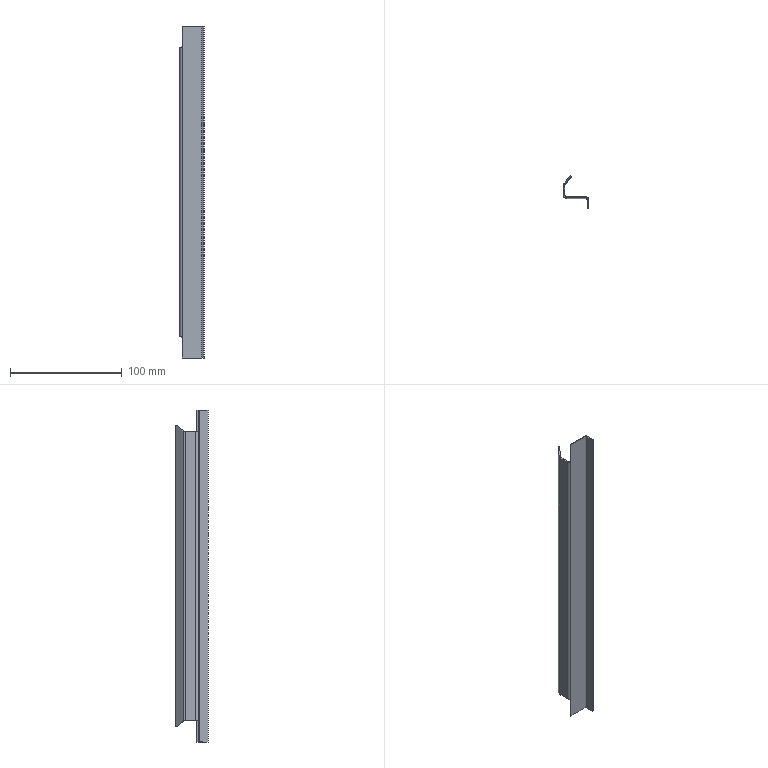Part | SolidWorks | features CombineBodies 1, FlatPattern 1, FlattenBends 1, ICE 1, MirrorStock 1, MoveCopyBody 1, ProcessBends 1, SheetMetal 1 | 1 solid | 34 faces | box 22.2 x 28.771 x 297.6 mm | volume 16962 mm3 | plane 28 | cylinder 6 | commonest cylinder face diameters 2 x3 4.4 x3
STEP:
#1=CARTESIAN_POINT('',(-28.126,247.,-284.107));
#2=VERTEX_POINT('',#1);
#3=CARTESIAN_POINT('',(-29.046,247.771,-284.107));
#4=VERTEX_POINT('',#3);
#5=CARTESIAN_POINT('',(385.778,-100.307,-284.107));
#6=DIRECTION('',(-0.766,0.6428,0.));
#7=VECTOR('',#6,1000.);
#8=LINE('',#5,#7);
#9=EDGE_CURVE('',#2,#4,#8,.T.);
#10=ORIENTED_EDGE('',*,*,#9,.T.);
#11=CARTESIAN_POINT('',(-29.046,247.771,-13.493));
#12=VERTEX_POINT('',#11);
#13=CARTESIAN_POINT('',(-29.046,247.771,-333.94));
#14=DIRECTION('',(0.,0.,1.));
#15=VECTOR('',#14,1000.);
#16=LINE('',#13,#15);
#17=EDGE_CURVE('',#4,#12,#16,.T.);
#18=ORIENTED_EDGE('',*,*,#17,.T.);
#19=CARTESIAN_POINT('',(-28.126,247.,-13.493));
#20=VERTEX_POINT('',#19);
#21=CARTESIAN_POINT('',(385.778,-100.307,-13.493));
#22=DIRECTION('',(-0.766,0.6428,0.));
#23=VECTOR('',#22,1000.);
#24=LINE('',#21,#23);
#25=EDGE_CURVE('',#20,#12,#24,.T.);
#26=ORIENTED_EDGE('',*,*,#25,.F.);
#27=CARTESIAN_POINT('',(-28.126,247.,-333.94));
#28=DIRECTION('',(0.,0.,1.));
#29=VECTOR('',#28,1000.);
#30=LINE('',#27,#29);
#31=EDGE_CURVE('',#2,#20,#30,.T.);
#32=ORIENTED_EDGE('',*,*,#31,.F.);
#33=EDGE_LOOP('',(#10,#18,#26,#32));
#34=FACE_OUTER_BOUND('',#33,.T.);
#35=CARTESIAN_POINT('',(385.778,-100.307,-333.94));
#36=DIRECTION('',(-0.6428,-0.766,0.));
#37=DIRECTION('',(0.766,-0.6428,0.));
#38=AXIS2_PLACEMENT_3D('',#35,#36,#37);
#39=PLANE('',#38);
#40=ADVANCED_FACE('',(#34),#39,.F.);
#41=CARTESIAN_POINT('',(-34.553,241.208,-19.));
#42=VERTEX_POINT('',#41);
#43=CARTESIAN_POINT('',(-122.736,136.115,-107.183));
#44=DIRECTION('',(0.5407,0.6444,0.5407));
#45=VECTOR('',#44,1000.);
#46=LINE('',#43,#45);
#47=EDGE_CURVE('',#42,#12,#46,.T.);
#48=ORIENTED_EDGE('',*,*,#47,.F.);
#49=CARTESIAN_POINT('',(-33.634,240.437,-19.));
#50=VERTEX_POINT('',#49);
#51=CARTESIAN_POINT('',(380.27,-106.87,-19.));
#52=DIRECTION('',(-0.766,0.6428,0.));
#53=VECTOR('',#52,1000.);
#54=LINE('',#51,#53);
#55=EDGE_CURVE('',#50,#42,#54,.T.);
#56=ORIENTED_EDGE('',*,*,#55,.F.);
#57=CARTESIAN_POINT('',(-121.817,135.344,-107.183));
#58=DIRECTION('',(0.5407,0.6444,0.5407));
#59=VECTOR('',#58,1000.);
#60=LINE('',#57,#59);
#61=EDGE_CURVE('',#50,#20,#60,.T.);
#62=ORIENTED_EDGE('',*,*,#61,.T.);
#63=ORIENTED_EDGE('',*,*,#25,.T.);
#64=EDGE_LOOP('',(#48,#56,#62,#63));
#65=FACE_OUTER_BOUND('',#64,.T.);
#66=CARTESIAN_POINT('',(292.087,-211.963,-107.183));
#67=DIRECTION('',(-0.3476,-0.4142,0.8412));
#68=DIRECTION('',(-0.5407,-0.6444,-0.5407));
#69=AXIS2_PLACEMENT_3D('',#66,#67,#68);
#70=PLANE('',#69);
#71=ADVANCED_FACE('',(#65),#70,.T.);
#72=CARTESIAN_POINT('',(-33.634,240.437,-278.6));
#73=VERTEX_POINT('',#72);
#74=CARTESIAN_POINT('',(-34.553,241.208,-278.6));
#75=VERTEX_POINT('',#74);
#76=CARTESIAN_POINT('',(380.27,-106.87,-278.6));
#77=DIRECTION('',(-0.766,0.6428,0.));
#78=VECTOR('',#77,1000.);
#79=LINE('',#76,#78);
#80=EDGE_CURVE('',#73,#75,#79,.T.);
#81=ORIENTED_EDGE('',*,*,#80,.T.);
#82=CARTESIAN_POINT('',(-14.476,265.135,-298.677));
#83=DIRECTION('',(0.5407,0.6444,-0.5407));
#84=VECTOR('',#83,1000.);
#85=LINE('',#82,#84);
#86=EDGE_CURVE('',#75,#4,#85,.T.);
#87=ORIENTED_EDGE('',*,*,#86,.T.);
#88=ORIENTED_EDGE('',*,*,#9,.F.);
#89=CARTESIAN_POINT('',(-13.556,264.364,-298.677));
#90=DIRECTION('',(0.5407,0.6444,-0.5407));
#91=VECTOR('',#90,1000.);
#92=LINE('',#89,#91);
#93=EDGE_CURVE('',#73,#2,#92,.T.);
#94=ORIENTED_EDGE('',*,*,#93,.F.);
#95=EDGE_LOOP('',(#81,#87,#88,#94));
#96=FACE_OUTER_BOUND('',#95,.T.);
#97=CARTESIAN_POINT('',(400.348,-82.943,-298.677));
#98=DIRECTION('',(0.3476,0.4142,0.8412));
#99=DIRECTION('',(-0.5407,-0.6444,0.5407));
#100=AXIS2_PLACEMENT_3D('',#97,#98,#99);
#101=PLANE('',#100);
#102=ADVANCED_FACE('',(#96),#101,.F.);
#103=CARTESIAN_POINT('',(-33.766,240.279,-278.6));
#104=VERTEX_POINT('',#103);
#105=CARTESIAN_POINT('',(-34.685,241.05,-278.6));
#106=VERTEX_POINT('',#105);
#107=CARTESIAN_POINT('',(380.138,-107.028,-278.6));
#108=DIRECTION('',(-0.766,0.6428,0.));
#109=VECTOR('',#108,1000.);
#110=LINE('',#107,#109);
#111=EDGE_CURVE('',#104,#106,#110,.T.);
#112=ORIENTED_EDGE('',*,*,#111,.T.);
#113=CARTESIAN_POINT('',(-29.046,247.771,-278.6));
#114=DIRECTION('',(0.6428,0.766,0.));
#115=VECTOR('',#114,1000.);
#116=LINE('',#113,#115);
#117=EDGE_CURVE('',#106,#75,#116,.T.);
#118=ORIENTED_EDGE('',*,*,#117,.T.);
#119=ORIENTED_EDGE('',*,*,#80,.F.);
#120=CARTESIAN_POINT('',(-28.126,247.,-278.6));
#121=DIRECTION('',(0.6428,0.766,0.));
#122=VECTOR('',#121,1000.);
#123=LINE('',#120,#122);
#124=EDGE_CURVE('',#104,#73,#123,.T.);
#125=ORIENTED_EDGE('',*,*,#124,.F.);
#126=EDGE_LOOP('',(#112,#118,#119,#125));
#127=FACE_OUTER_BOUND('',#126,.T.);
#128=CARTESIAN_POINT('',(385.778,-100.307,-278.6));
#129=DIRECTION('',(0.,0.,1.));
#130=DIRECTION('',(-0.6428,-0.766,0.));
#131=AXIS2_PLACEMENT_3D('',#128,#129,#130);
#132=PLANE('',#131);
#133=ADVANCED_FACE('',(#127),#132,.F.);
#134=ORIENTED_EDGE('',*,*,#86,.F.);
#135=ORIENTED_EDGE('',*,*,#117,.F.);
#136=CARTESIAN_POINT('',(-34.685,241.05,-19.));
#137=VERTEX_POINT('',#136);
#138=CARTESIAN_POINT('',(-34.685,241.05,-333.94));
#139=DIRECTION('',(0.,0.,1.));
#140=VECTOR('',#139,1000.);
#141=LINE('',#138,#140);
#142=EDGE_CURVE('',#106,#137,#141,.T.);
#143=ORIENTED_EDGE('',*,*,#142,.T.);
#144=CARTESIAN_POINT('',(-29.046,247.771,-19.));
#145=DIRECTION('',(0.6428,0.766,0.));
#146=VECTOR('',#145,1000.);
#147=LINE('',#144,#146);
#148=EDGE_CURVE('',#137,#42,#147,.T.);
#149=ORIENTED_EDGE('',*,*,#148,.T.);
#150=ORIENTED_EDGE('',*,*,#47,.T.);
#151=ORIENTED_EDGE('',*,*,#17,.F.);
#152=EDGE_LOOP('',(#134,#135,#143,#149,#150,#151));
#153=FACE_OUTER_BOUND('',#152,.T.);
#154=CARTESIAN_POINT('',(-29.046,247.771,-333.94));
#155=DIRECTION('',(0.766,-0.6428,0.));
#156=DIRECTION('',(0.6428,0.766,0.));
#157=AXIS2_PLACEMENT_3D('',#154,#155,#156);
#158=PLANE('',#157);
#159=ADVANCED_FACE('',(#153),#158,.F.);
#160=ORIENTED_EDGE('',*,*,#148,.F.);
#161=CARTESIAN_POINT('',(-33.766,240.279,-19.));
#162=VERTEX_POINT('',#161);
#163=CARTESIAN_POINT('',(380.138,-107.028,-19.));
#164=DIRECTION('',(-0.766,0.6428,0.));
#165=VECTOR('',#164,1000.);
#166=LINE('',#163,#165);
#167=EDGE_CURVE('',#162,#137,#166,.T.);
#168=ORIENTED_EDGE('',*,*,#167,.F.);
#169=CARTESIAN_POINT('',(-28.126,247.,-19.));
#170=DIRECTION('',(0.6428,0.766,0.));
#171=VECTOR('',#170,1000.);
#172=LINE('',#169,#171);
#173=EDGE_CURVE('',#162,#50,#172,.T.);
#174=ORIENTED_EDGE('',*,*,#173,.T.);
#175=ORIENTED_EDGE('',*,*,#55,.T.);
#176=EDGE_LOOP('',(#160,#168,#174,#175));
#177=FACE_OUTER_BOUND('',#176,.T.);
#178=CARTESIAN_POINT('',(385.778,-100.307,-19.));
#179=DIRECTION('',(0.,0.,1.));
#180=DIRECTION('',(-0.6428,-0.766,0.));
#181=AXIS2_PLACEMENT_3D('',#178,#179,#180);
#182=PLANE('',#181);
#183=ADVANCED_FACE('',(#177),#182,.T.);
#184=ORIENTED_EDGE('',*,*,#31,.T.);
#185=ORIENTED_EDGE('',*,*,#61,.F.);
#186=ORIENTED_EDGE('',*,*,#173,.F.);
#187=CARTESIAN_POINT('',(-33.766,240.279,-333.94));
#188=DIRECTION('',(0.,0.,1.));
#189=VECTOR('',#188,1000.);
#190=LINE('',#187,#189);
#191=EDGE_CURVE('',#104,#162,#190,.T.);
#192=ORIENTED_EDGE('',*,*,#191,.F.);
#193=ORIENTED_EDGE('',*,*,#124,.T.);
#194=ORIENTED_EDGE('',*,*,#93,.T.);
#195=EDGE_LOOP('',(#184,#185,#186,#192,#193,#194));
#196=FACE_OUTER_BOUND('',#195,.T.);
#197=CARTESIAN_POINT('',(-28.126,247.,-333.94));
#198=DIRECTION('',(0.766,-0.6428,0.));
#199=DIRECTION('',(0.6428,0.766,0.));
#200=AXIS2_PLACEMENT_3D('',#197,#198,#199);
#201=PLANE('',#200);
#202=ADVANCED_FACE('',(#196),#201,.T.);
#203=CARTESIAN_POINT('',(-34.,230.,-278.6));
#204=VERTEX_POINT('',#203);
#205=CARTESIAN_POINT('',(-35.2,230.,-278.6));
#206=VERTEX_POINT('',#205);
#207=CARTESIAN_POINT('',(484.358,230.,-278.6));
#208=DIRECTION('',(-1.,0.,0.));
#209=VECTOR('',#208,1000.);
#210=LINE('',#207,#209);
#211=EDGE_CURVE('',#204,#206,#210,.T.);
#212=ORIENTED_EDGE('',*,*,#211,.T.);
#213=CARTESIAN_POINT('',(-35.2,239.636,-278.6));
#214=VERTEX_POINT('',#213);
#215=CARTESIAN_POINT('',(-35.2,240.,-278.6));
#216=DIRECTION('',(0.,1.,0.));
#217=VECTOR('',#216,1000.);
#218=LINE('',#215,#217);
#219=EDGE_CURVE('',#206,#214,#218,.T.);
#220=ORIENTED_EDGE('',*,*,#219,.T.);
#221=CARTESIAN_POINT('',(-34.,239.636,-278.6));
#222=VERTEX_POINT('',#221);
#223=CARTESIAN_POINT('',(484.358,239.636,-278.6));
#224=DIRECTION('',(-1.,0.,0.));
#225=VECTOR('',#224,1000.);
#226=LINE('',#223,#225);
#227=EDGE_CURVE('',#222,#214,#226,.T.);
#228=ORIENTED_EDGE('',*,*,#227,.F.);
#229=CARTESIAN_POINT('',(-34.,240.,-278.6));
#230=DIRECTION('',(0.,1.,0.));
#231=VECTOR('',#230,1000.);
#232=LINE('',#229,#231);
#233=EDGE_CURVE('',#204,#222,#232,.T.);
#234=ORIENTED_EDGE('',*,*,#233,.F.);
#235=EDGE_LOOP('',(#212,#220,#228,#234));
#236=FACE_OUTER_BOUND('',#235,.T.);
#237=CARTESIAN_POINT('',(484.358,240.,-278.6));
#238=DIRECTION('',(0.,0.,1.));
#239=DIRECTION('',(1.,0.,0.));
#240=AXIS2_PLACEMENT_3D('',#237,#238,#239);
#241=PLANE('',#240);
#242=ADVANCED_FACE('',(#236),#241,.F.);
#243=ORIENTED_EDGE('',*,*,#219,.F.);
#244=CARTESIAN_POINT('',(-35.2,230.,-19.));
#245=VERTEX_POINT('',#244);
#246=CARTESIAN_POINT('',(-35.2,230.,-333.94));
#247=DIRECTION('',(0.,0.,1.));
#248=VECTOR('',#247,1000.);
#249=LINE('',#246,#248);
#250=EDGE_CURVE('',#206,#245,#249,.T.);
#251=ORIENTED_EDGE('',*,*,#250,.T.);
#252=CARTESIAN_POINT('',(-35.2,239.636,-19.));
#253=VERTEX_POINT('',#252);
#254=CARTESIAN_POINT('',(-35.2,240.,-19.));
#255=DIRECTION('',(0.,1.,0.));
#256=VECTOR('',#255,1000.);
#257=LINE('',#254,#256);
#258=EDGE_CURVE('',#245,#253,#257,.T.);
#259=ORIENTED_EDGE('',*,*,#258,.T.);
#260=CARTESIAN_POINT('',(-35.2,239.636,-333.94));
#261=DIRECTION('',(0.,0.,1.));
#262=VECTOR('',#261,1000.);
#263=LINE('',#260,#262);
#264=EDGE_CURVE('',#214,#253,#263,.T.);
#265=ORIENTED_EDGE('',*,*,#264,.F.);
#266=EDGE_LOOP('',(#243,#251,#259,#265));
#267=FACE_OUTER_BOUND('',#266,.T.);
#268=CARTESIAN_POINT('',(-35.2,240.,-333.94));
#269=DIRECTION('',(1.,0.,0.));
#270=DIRECTION('',(0.,0.,1.));
#271=AXIS2_PLACEMENT_3D('',#268,#269,#270);
#272=PLANE('',#271);
#273=ADVANCED_FACE('',(#267),#272,.F.);
#274=ORIENTED_EDGE('',*,*,#258,.F.);
#275=CARTESIAN_POINT('',(-34.,230.,-19.));
#276=VERTEX_POINT('',#275);
#277=CARTESIAN_POINT('',(484.358,230.,-19.));
#278=DIRECTION('',(-1.,0.,0.));
#279=VECTOR('',#278,1000.);
#280=LINE('',#277,#279);
#281=EDGE_CURVE('',#276,#245,#280,.T.);
#282=ORIENTED_EDGE('',*,*,#281,.F.);
#283=CARTESIAN_POINT('',(-34.,239.636,-19.));
#284=VERTEX_POINT('',#283);
#285=CARTESIAN_POINT('',(-34.,240.,-19.));
#286=DIRECTION('',(0.,1.,0.));
#287=VECTOR('',#286,1000.);
#288=LINE('',#285,#287);
#289=EDGE_CURVE('',#276,#284,#288,.T.);
#290=ORIENTED_EDGE('',*,*,#289,.T.);
#291=CARTESIAN_POINT('',(484.358,239.636,-19.));
#292=DIRECTION('',(-1.,0.,0.));
#293=VECTOR('',#292,1000.);
#294=LINE('',#291,#293);
#295=EDGE_CURVE('',#284,#253,#294,.T.);
#296=ORIENTED_EDGE('',*,*,#295,.T.);
#297=EDGE_LOOP('',(#274,#282,#290,#296));
#298=FACE_OUTER_BOUND('',#297,.T.);
#299=CARTESIAN_POINT('',(484.358,240.,-19.));
#300=DIRECTION('',(0.,0.,1.));
#301=DIRECTION('',(0.,-1.,0.));
#302=AXIS2_PLACEMENT_3D('',#299,#300,#301);
#303=PLANE('',#302);
#304=ADVANCED_FACE('',(#298),#303,.T.);
#305=CARTESIAN_POINT('',(-34.,239.636,-333.94));
#306=DIRECTION('',(0.,0.,1.));
#307=VECTOR('',#306,1000.);
#308=LINE('',#305,#307);
#309=EDGE_CURVE('',#222,#284,#308,.T.);
#310=ORIENTED_EDGE('',*,*,#309,.T.);
#311=ORIENTED_EDGE('',*,*,#289,.F.);
#312=CARTESIAN_POINT('',(-34.,230.,-333.94));
#313=DIRECTION('',(0.,0.,1.));
#314=VECTOR('',#313,1000.);
#315=LINE('',#312,#314);
#316=EDGE_CURVE('',#204,#276,#315,.T.);
#317=ORIENTED_EDGE('',*,*,#316,.F.);
#318=ORIENTED_EDGE('',*,*,#233,.T.);
#319=EDGE_LOOP('',(#310,#311,#317,#318));
#320=FACE_OUTER_BOUND('',#319,.T.);
#321=CARTESIAN_POINT('',(-34.,240.,-333.94));
#322=DIRECTION('',(1.,0.,0.));
#323=DIRECTION('',(0.,0.,1.));
#324=AXIS2_PLACEMENT_3D('',#321,#322,#323);
#325=PLANE('',#324);
#326=ADVANCED_FACE('',(#320),#325,.T.);
#327=CARTESIAN_POINT('',(-33.,229.,-297.6));
#328=VERTEX_POINT('',#327);
#329=CARTESIAN_POINT('',(-33.,229.,-278.6));
#330=VERTEX_POINT('',#329);
#331=CARTESIAN_POINT('',(-33.,229.,-333.94));
#332=DIRECTION('',(0.,0.,1.));
#333=VECTOR('',#332,1000.);
#334=LINE('',#331,#333);
#335=EDGE_CURVE('',#328,#330,#334,.T.);
#336=ORIENTED_EDGE('',*,*,#335,.T.);
#337=CARTESIAN_POINT('',(-33.,229.,-19.));
#338=VERTEX_POINT('',#337);
#339=CARTESIAN_POINT('',(-33.,229.,-333.94));
#340=DIRECTION('',(0.,0.,1.));
#341=VECTOR('',#340,1000.);
#342=LINE('',#339,#341);
#343=EDGE_CURVE('',#330,#338,#342,.T.);
#344=ORIENTED_EDGE('',*,*,#343,.T.);
#345=CARTESIAN_POINT('',(-33.,229.,0.));
#346=VERTEX_POINT('',#345);
#347=CARTESIAN_POINT('',(-33.,229.,148.811));
#348=DIRECTION('',(0.,0.,-1.));
#349=VECTOR('',#348,1000.);
#350=LINE('',#347,#349);
#351=EDGE_CURVE('',#346,#338,#350,.T.);
#352=ORIENTED_EDGE('',*,*,#351,.F.);
#353=CARTESIAN_POINT('',(-15.2,229.,0.));
#354=VERTEX_POINT('',#353);
#355=CARTESIAN_POINT('',(-34.,229.,0.));
#356=DIRECTION('',(1.,0.,0.));
#357=VECTOR('',#356,1000.);
#358=LINE('',#355,#357);
#359=EDGE_CURVE('',#346,#354,#358,.T.);
#360=ORIENTED_EDGE('',*,*,#359,.T.);
#361=CARTESIAN_POINT('',(-15.2,229.,-297.6));
#362=VERTEX_POINT('',#361);
#363=CARTESIAN_POINT('',(-15.2,229.,-333.94));
#364=DIRECTION('',(0.,0.,1.));
#365=VECTOR('',#364,1000.);
#366=LINE('',#363,#365);
#367=EDGE_CURVE('',#362,#354,#366,.T.);
#368=ORIENTED_EDGE('',*,*,#367,.F.);
#369=CARTESIAN_POINT('',(-34.,229.,-297.6));
#370=DIRECTION('',(1.,0.,0.));
#371=VECTOR('',#370,1000.);
#372=LINE('',#369,#371);
#373=EDGE_CURVE('',#328,#362,#372,.T.);
#374=ORIENTED_EDGE('',*,*,#373,.F.);
#375=EDGE_LOOP('',(#336,#344,#352,#360,#368,#374));
#376=FACE_OUTER_BOUND('',#375,.T.);
#377=CARTESIAN_POINT('',(-34.,229.,-333.94));
#378=DIRECTION('',(0.,1.,0.));
#379=DIRECTION('',(0.,0.,-1.));
#380=AXIS2_PLACEMENT_3D('',#377,#378,#379);
#381=PLANE('',#380);
#382=ADVANCED_FACE('',(#376),#381,.T.);
#383=ORIENTED_EDGE('',*,*,#373,.T.);
#384=CARTESIAN_POINT('',(-15.2,227.8,-297.6));
#385=VERTEX_POINT('',#384);
#386=CARTESIAN_POINT('',(-15.2,-368.464,-297.6));
#387=DIRECTION('',(0.,1.,0.));
#388=VECTOR('',#387,1000.);
#389=LINE('',#386,#388);
#390=EDGE_CURVE('',#385,#362,#389,.T.);
#391=ORIENTED_EDGE('',*,*,#390,.F.);
#392=CARTESIAN_POINT('',(-33.,227.8,-297.6));
#393=VERTEX_POINT('',#392);
#394=CARTESIAN_POINT('',(-34.,227.8,-297.6));
#395=DIRECTION('',(1.,0.,0.));
#396=VECTOR('',#395,1000.);
#397=LINE('',#394,#396);
#398=EDGE_CURVE('',#393,#385,#397,.T.);
#399=ORIENTED_EDGE('',*,*,#398,.F.);
#400=CARTESIAN_POINT('',(-33.,-368.464,-297.6));
#401=DIRECTION('',(0.,1.,0.));
#402=VECTOR('',#401,1000.);
#403=LINE('',#400,#402);
#404=EDGE_CURVE('',#393,#328,#403,.T.);
#405=ORIENTED_EDGE('',*,*,#404,.T.);
#406=EDGE_LOOP('',(#383,#391,#399,#405));
#407=FACE_OUTER_BOUND('',#406,.T.);
#408=CARTESIAN_POINT('',(-34.,-368.464,-297.6));
#409=DIRECTION('',(0.,0.,1.));
#410=DIRECTION('',(0.,1.,0.));
#411=AXIS2_PLACEMENT_3D('',#408,#409,#410);
#412=PLANE('',#411);
#413=ADVANCED_FACE('',(#407),#412,.F.);
#414=CARTESIAN_POINT('',(-15.2,227.8,0.));
#415=VERTEX_POINT('',#414);
#416=CARTESIAN_POINT('',(-15.2,-368.464,0.));
#417=DIRECTION('',(0.,1.,0.));
#418=VECTOR('',#417,1000.);
#419=LINE('',#416,#418);
#420=EDGE_CURVE('',#415,#354,#419,.T.);
#421=ORIENTED_EDGE('',*,*,#420,.T.);
#422=ORIENTED_EDGE('',*,*,#359,.F.);
#423=CARTESIAN_POINT('',(-33.,227.8,0.));
#424=VERTEX_POINT('',#423);
#425=CARTESIAN_POINT('',(-33.,-368.464,0.));
#426=DIRECTION('',(0.,1.,0.));
#427=VECTOR('',#426,1000.);
#428=LINE('',#425,#427);
#429=EDGE_CURVE('',#424,#346,#428,.T.);
#430=ORIENTED_EDGE('',*,*,#429,.F.);
#431=CARTESIAN_POINT('',(-34.,227.8,0.));
#432=DIRECTION('',(1.,0.,0.));
#433=VECTOR('',#432,1000.);
#434=LINE('',#431,#433);
#435=EDGE_CURVE('',#424,#415,#434,.T.);
#436=ORIENTED_EDGE('',*,*,#435,.T.);
#437=EDGE_LOOP('',(#421,#422,#430,#436));
#438=FACE_OUTER_BOUND('',#437,.T.);
#439=CARTESIAN_POINT('',(-34.,-368.464,0.));
#440=DIRECTION('',(0.,0.,1.));
#441=DIRECTION('',(0.,1.,0.));
#442=AXIS2_PLACEMENT_3D('',#439,#440,#441);
#443=PLANE('',#442);
#444=ADVANCED_FACE('',(#438),#443,.T.);
#445=ORIENTED_EDGE('',*,*,#351,.T.);
#446=CARTESIAN_POINT('',(-33.,227.8,-19.));
#447=VERTEX_POINT('',#446);
#448=CARTESIAN_POINT('',(-33.,-368.464,-19.));
#449=DIRECTION('',(0.,1.,0.));
#450=VECTOR('',#449,1000.);
#451=LINE('',#448,#450);
#452=EDGE_CURVE('',#447,#338,#451,.T.);
#453=ORIENTED_EDGE('',*,*,#452,.F.);
#454=CARTESIAN_POINT('',(-33.,227.8,148.811));
#455=DIRECTION('',(0.,0.,-1.));
#456=VECTOR('',#455,1000.);
#457=LINE('',#454,#456);
#458=EDGE_CURVE('',#424,#447,#457,.T.);
#459=ORIENTED_EDGE('',*,*,#458,.F.);
#460=ORIENTED_EDGE('',*,*,#429,.T.);
#461=EDGE_LOOP('',(#445,#453,#459,#460));
#462=FACE_OUTER_BOUND('',#461,.T.);
#463=CARTESIAN_POINT('',(-33.,-368.464,148.811));
#464=DIRECTION('',(1.,0.,0.));
#465=DIRECTION('',(0.,1.,0.));
#466=AXIS2_PLACEMENT_3D('',#463,#464,#465);
#467=PLANE('',#466);
#468=ADVANCED_FACE('',(#462),#467,.F.);
#469=CARTESIAN_POINT('',(-33.,227.8,-278.6));
#470=VERTEX_POINT('',#469);
#471=CARTESIAN_POINT('',(-33.,-368.464,-278.6));
#472=DIRECTION('',(0.,1.,0.));
#473=VECTOR('',#472,1000.);
#474=LINE('',#471,#473);
#475=EDGE_CURVE('',#470,#330,#474,.T.);
#476=ORIENTED_EDGE('',*,*,#475,.T.);
#477=ORIENTED_EDGE('',*,*,#335,.F.);
#478=ORIENTED_EDGE('',*,*,#404,.F.);
#479=CARTESIAN_POINT('',(-33.,227.8,-333.94));
#480=DIRECTION('',(0.,0.,1.));
#481=VECTOR('',#480,1000.);
#482=LINE('',#479,#481);
#483=EDGE_CURVE('',#393,#470,#482,.T.);
#484=ORIENTED_EDGE('',*,*,#483,.T.);
#485=EDGE_LOOP('',(#476,#477,#478,#484));
#486=FACE_OUTER_BOUND('',#485,.T.);
#487=CARTESIAN_POINT('',(-33.,-368.464,-333.94));
#488=DIRECTION('',(-1.,0.,0.));
#489=DIRECTION('',(0.,-1.,0.));
#490=AXIS2_PLACEMENT_3D('',#487,#488,#489);
#491=PLANE('',#490);
#492=ADVANCED_FACE('',(#486),#491,.T.);
#493=ORIENTED_EDGE('',*,*,#398,.T.);
#494=CARTESIAN_POINT('',(-15.2,227.8,-333.94));
#495=DIRECTION('',(0.,0.,1.));
#496=VECTOR('',#495,1000.);
#497=LINE('',#494,#496);
#498=EDGE_CURVE('',#385,#415,#497,.T.);
#499=ORIENTED_EDGE('',*,*,#498,.T.);
#500=ORIENTED_EDGE('',*,*,#435,.F.);
#501=ORIENTED_EDGE('',*,*,#458,.T.);
#502=CARTESIAN_POINT('',(-33.,227.8,-333.94));
#503=DIRECTION('',(0.,0.,1.));
#504=VECTOR('',#503,1000.);
#505=LINE('',#502,#504);
#506=EDGE_CURVE('',#470,#447,#505,.T.);
#507=ORIENTED_EDGE('',*,*,#506,.F.);
#508=ORIENTED_EDGE('',*,*,#483,.F.);
#509=EDGE_LOOP('',(#493,#499,#500,#501,#507,#508));
#510=FACE_OUTER_BOUND('',#509,.T.);
#511=CARTESIAN_POINT('',(-34.,227.8,-333.94));
#512=DIRECTION('',(0.,1.,0.));
#513=DIRECTION('',(0.,0.,-1.));
#514=AXIS2_PLACEMENT_3D('',#511,#512,#513);
#515=PLANE('',#514);
#516=ADVANCED_FACE('',(#510),#515,.F.);
#517=CARTESIAN_POINT('',(-13.,219.,-297.6));
#518=VERTEX_POINT('',#517);
#519=CARTESIAN_POINT('',(-13.,219.,0.));
#520=VERTEX_POINT('',#519);
#521=CARTESIAN_POINT('',(-13.,219.,-333.94));
#522=DIRECTION('',(0.,0.,1.));
#523=VECTOR('',#522,1000.);
#524=LINE('',#521,#523);
#525=EDGE_CURVE('',#518,#520,#524,.T.);
#526=ORIENTED_EDGE('',*,*,#525,.T.);
#527=CARTESIAN_POINT('',(-14.2,219.,0.));
#528=VERTEX_POINT('',#527);
#529=CARTESIAN_POINT('',(-609.604,219.,0.));
#530=DIRECTION('',(1.,0.,0.));
#531=VECTOR('',#530,1000.);
#532=LINE('',#529,#531);
#533=EDGE_CURVE('',#528,#520,#532,.T.);
#534=ORIENTED_EDGE('',*,*,#533,.F.);
#535=CARTESIAN_POINT('',(-14.2,219.,-297.6));
#536=VERTEX_POINT('',#535);
#537=CARTESIAN_POINT('',(-14.2,219.,-333.94));
#538=DIRECTION('',(0.,0.,1.));
#539=VECTOR('',#538,1000.);
#540=LINE('',#537,#539);
#541=EDGE_CURVE('',#536,#528,#540,.T.);
#542=ORIENTED_EDGE('',*,*,#541,.F.);
#543=CARTESIAN_POINT('',(-609.604,219.,-297.6));
#544=DIRECTION('',(1.,0.,0.));
#545=VECTOR('',#544,1000.);
#546=LINE('',#543,#545);
#547=EDGE_CURVE('',#536,#518,#546,.T.);
#548=ORIENTED_EDGE('',*,*,#547,.T.);
#549=EDGE_LOOP('',(#526,#534,#542,#548));
#550=FACE_OUTER_BOUND('',#549,.T.);
#551=CARTESIAN_POINT('',(-609.604,219.,-333.94));
#552=DIRECTION('',(0.,1.,0.));
#553=DIRECTION('',(-1.,0.,0.));
#554=AXIS2_PLACEMENT_3D('',#551,#552,#553);
#555=PLANE('',#554);
#556=ADVANCED_FACE('',(#550),#555,.F.);
#557=CARTESIAN_POINT('',(-14.2,226.8,-297.6));
#558=VERTEX_POINT('',#557);
#559=CARTESIAN_POINT('',(-14.2,229.,-297.6));
#560=DIRECTION('',(0.,-1.,0.));
#561=VECTOR('',#560,1000.);
#562=LINE('',#559,#561);
#563=EDGE_CURVE('',#558,#536,#562,.T.);
#564=ORIENTED_EDGE('',*,*,#563,.T.);
#565=ORIENTED_EDGE('',*,*,#541,.T.);
#566=CARTESIAN_POINT('',(-14.2,226.8,0.));
#567=VERTEX_POINT('',#566);
#568=CARTESIAN_POINT('',(-14.2,229.,0.));
#569=DIRECTION('',(0.,-1.,0.));
#570=VECTOR('',#569,1000.);
#571=LINE('',#568,#570);
#572=EDGE_CURVE('',#567,#528,#571,.T.);
#573=ORIENTED_EDGE('',*,*,#572,.F.);
#574=CARTESIAN_POINT('',(-14.2,226.8,-333.94));
#575=DIRECTION('',(0.,0.,1.));
#576=VECTOR('',#575,1000.);
#577=LINE('',#574,#576);
#578=EDGE_CURVE('',#558,#567,#577,.T.);
#579=ORIENTED_EDGE('',*,*,#578,.F.);
#580=EDGE_LOOP('',(#564,#565,#573,#579));
#581=FACE_OUTER_BOUND('',#580,.T.);
#582=CARTESIAN_POINT('',(-14.2,229.,-333.94));
#583=DIRECTION('',(1.,0.,0.));
#584=DIRECTION('',(0.,1.,0.));
#585=AXIS2_PLACEMENT_3D('',#582,#583,#584);
#586=PLANE('',#585);
#587=ADVANCED_FACE('',(#581),#586,.F.);
#588=CARTESIAN_POINT('',(-13.,226.8,-297.6));
#589=VERTEX_POINT('',#588);
#590=CARTESIAN_POINT('',(-13.,229.,-297.6));
#591=DIRECTION('',(0.,-1.,0.));
#592=VECTOR('',#591,1000.);
#593=LINE('',#590,#592);
#594=EDGE_CURVE('',#589,#518,#593,.T.);
#595=ORIENTED_EDGE('',*,*,#594,.T.);
#596=ORIENTED_EDGE('',*,*,#547,.F.);
#597=ORIENTED_EDGE('',*,*,#563,.F.);
#598=CARTESIAN_POINT('',(-609.604,226.8,-297.6));
#599=DIRECTION('',(1.,0.,0.));
#600=VECTOR('',#599,1000.);
#601=LINE('',#598,#600);
#602=EDGE_CURVE('',#558,#589,#601,.T.);
#603=ORIENTED_EDGE('',*,*,#602,.T.);
#604=EDGE_LOOP('',(#595,#596,#597,#603));
#605=FACE_OUTER_BOUND('',#604,.T.);
#606=CARTESIAN_POINT('',(-609.604,229.,-297.6));
#607=DIRECTION('',(0.,0.,1.));
#608=DIRECTION('',(1.,0.,0.));
#609=AXIS2_PLACEMENT_3D('',#606,#607,#608);
#610=PLANE('',#609);
#611=ADVANCED_FACE('',(#605),#610,.F.);
#612=CARTESIAN_POINT('',(-13.,226.8,0.));
#613=VERTEX_POINT('',#612);
#614=CARTESIAN_POINT('',(-13.,226.8,-333.94));
#615=DIRECTION('',(0.,0.,1.));
#616=VECTOR('',#615,1000.);
#617=LINE('',#614,#616);
#618=EDGE_CURVE('',#589,#613,#617,.T.);
#619=ORIENTED_EDGE('',*,*,#618,.T.);
#620=CARTESIAN_POINT('',(-13.,229.,0.));
#621=DIRECTION('',(0.,-1.,0.));
#622=VECTOR('',#621,1000.);
#623=LINE('',#620,#622);
#624=EDGE_CURVE('',#613,#520,#623,.T.);
#625=ORIENTED_EDGE('',*,*,#624,.T.);
#626=ORIENTED_EDGE('',*,*,#525,.F.);
#627=ORIENTED_EDGE('',*,*,#594,.F.);
#628=EDGE_LOOP('',(#619,#625,#626,#627));
#629=FACE_OUTER_BOUND('',#628,.T.);
#630=CARTESIAN_POINT('',(-13.,229.,-333.94));
#631=DIRECTION('',(1.,0.,0.));
#632=DIRECTION('',(0.,1.,0.));
#633=AXIS2_PLACEMENT_3D('',#630,#631,#632);
#634=PLANE('',#633);
#635=ADVANCED_FACE('',(#629),#634,.T.);
#636=ORIENTED_EDGE('',*,*,#533,.T.);
#637=ORIENTED_EDGE('',*,*,#624,.F.);
#638=CARTESIAN_POINT('',(-609.604,226.8,0.));
#639=DIRECTION('',(1.,0.,0.));
#640=VECTOR('',#639,1000.);
#641=LINE('',#638,#640);
#642=EDGE_CURVE('',#567,#613,#641,.T.);
#643=ORIENTED_EDGE('',*,*,#642,.F.);
#644=ORIENTED_EDGE('',*,*,#572,.T.);
#645=EDGE_LOOP('',(#636,#637,#643,#644));
#646=FACE_OUTER_BOUND('',#645,.T.);
#647=CARTESIAN_POINT('',(-609.604,229.,0.));
#648=DIRECTION('',(0.,0.,1.));
#649=DIRECTION('',(1.,0.,0.));
#650=AXIS2_PLACEMENT_3D('',#647,#648,#649);
#651=PLANE('',#650);
#652=ADVANCED_FACE('',(#646),#651,.T.);
#653=ORIENTED_EDGE('',*,*,#420,.F.);
#654=CARTESIAN_POINT('',(-15.2,226.8,0.));
#655=DIRECTION('',(0.,0.,-1.));
#656=DIRECTION('',(-1.,0.,0.));
#657=AXIS2_PLACEMENT_3D('',#654,#655,#656);
#658=CIRCLE('',#657,1.);
#659=EDGE_CURVE('',#415,#567,#658,.T.);
#660=ORIENTED_EDGE('',*,*,#659,.T.);
#661=ORIENTED_EDGE('',*,*,#642,.T.);
#662=CARTESIAN_POINT('',(-15.2,226.8,0.));
#663=DIRECTION('',(0.,0.,-1.));
#664=DIRECTION('',(-1.,0.,0.));
#665=AXIS2_PLACEMENT_3D('',#662,#663,#664);
#666=CIRCLE('',#665,2.2);
#667=EDGE_CURVE('',#354,#613,#666,.T.);
#668=ORIENTED_EDGE('',*,*,#667,.F.);
#669=EDGE_LOOP('',(#653,#660,#661,#668));
#670=FACE_OUTER_BOUND('',#669,.T.);
#671=CARTESIAN_POINT('',(-15.2,226.8,0.));
#672=DIRECTION('',(0.,0.,1.));
#673=DIRECTION('',(1.,0.,0.));
#674=AXIS2_PLACEMENT_3D('',#671,#672,#673);
#675=PLANE('',#674);
#676=ADVANCED_FACE('',(#670),#675,.T.);
#677=ORIENTED_EDGE('',*,*,#618,.F.);
#678=CARTESIAN_POINT('',(-15.2,226.8,-297.6));
#679=DIRECTION('',(0.,0.,1.));
#680=DIRECTION('',(-1.,0.,0.));
#681=AXIS2_PLACEMENT_3D('',#678,#679,#680);
#682=CIRCLE('',#681,2.2);
#683=EDGE_CURVE('',#589,#362,#682,.T.);
#684=ORIENTED_EDGE('',*,*,#683,.T.);
#685=ORIENTED_EDGE('',*,*,#367,.T.);
#686=ORIENTED_EDGE('',*,*,#667,.T.);
#687=EDGE_LOOP('',(#677,#684,#685,#686));
#688=FACE_OUTER_BOUND('',#687,.T.);
#689=CARTESIAN_POINT('',(-15.2,226.8,301.685));
#690=DIRECTION('',(0.,0.,-1.));
#691=DIRECTION('',(-1.,0.,0.));
#692=AXIS2_PLACEMENT_3D('',#689,#690,#691);
#693=CYLINDRICAL_SURFACE('',#692,2.2);
#694=ADVANCED_FACE('',(#688),#693,.T.);
#695=CARTESIAN_POINT('',(-15.2,226.8,-297.6));
#696=DIRECTION('',(0.,0.,1.));
#697=DIRECTION('',(-1.,0.,0.));
#698=AXIS2_PLACEMENT_3D('',#695,#696,#697);
#699=CIRCLE('',#698,1.);
#700=EDGE_CURVE('',#558,#385,#699,.T.);
#701=ORIENTED_EDGE('',*,*,#700,.T.);
#702=ORIENTED_EDGE('',*,*,#390,.T.);
#703=ORIENTED_EDGE('',*,*,#683,.F.);
#704=ORIENTED_EDGE('',*,*,#602,.F.);
#705=EDGE_LOOP('',(#701,#702,#703,#704));
#706=FACE_OUTER_BOUND('',#705,.T.);
#707=CARTESIAN_POINT('',(-15.2,226.8,-297.6));
#708=DIRECTION('',(0.,0.,-1.));
#709=DIRECTION('',(-1.,0.,0.));
#710=AXIS2_PLACEMENT_3D('',#707,#708,#709);
#711=PLANE('',#710);
#712=ADVANCED_FACE('',(#706),#711,.T.);
#713=ORIENTED_EDGE('',*,*,#578,.T.);
#714=ORIENTED_EDGE('',*,*,#659,.F.);
#715=ORIENTED_EDGE('',*,*,#498,.F.);
#716=ORIENTED_EDGE('',*,*,#700,.F.);
#717=EDGE_LOOP('',(#713,#714,#715,#716));
#718=FACE_OUTER_BOUND('',#717,.T.);
#719=CARTESIAN_POINT('',(-15.2,226.8,301.685));
#720=DIRECTION('',(0.,0.,-1.));
#721=DIRECTION('',(-1.,0.,0.));
#722=AXIS2_PLACEMENT_3D('',#719,#720,#721);
#723=CYLINDRICAL_SURFACE('',#722,1.);
#724=ADVANCED_FACE('',(#718),#723,.F.);
#725=ORIENTED_EDGE('',*,*,#452,.T.);
#726=CARTESIAN_POINT('',(-33.,230.,-19.));
#727=DIRECTION('',(0.,0.,1.));
#728=DIRECTION('',(0.,-1.,0.));
#729=AXIS2_PLACEMENT_3D('',#726,#727,#728);
#730=CIRCLE('',#729,1.);
#731=EDGE_CURVE('',#276,#338,#730,.T.);
#732=ORIENTED_EDGE('',*,*,#731,.F.);
#733=ORIENTED_EDGE('',*,*,#281,.T.);
#734=CARTESIAN_POINT('',(-33.,230.,-19.));
#735=DIRECTION('',(0.,0.,1.));
#736=DIRECTION('',(0.,-1.,0.));
#737=AXIS2_PLACEMENT_3D('',#734,#735,#736);
#738=CIRCLE('',#737,2.2);
#739=EDGE_CURVE('',#245,#447,#738,.T.);
#740=ORIENTED_EDGE('',*,*,#739,.T.);
#741=EDGE_LOOP('',(#725,#732,#733,#740));
#742=FACE_OUTER_BOUND('',#741,.T.);
#743=CARTESIAN_POINT('',(-33.,230.,-19.));
#744=DIRECTION('',(0.,0.,-1.));
#745=DIRECTION('',(-1.,0.,0.));
#746=AXIS2_PLACEMENT_3D('',#743,#744,#745);
#747=PLANE('',#746);
#748=ADVANCED_FACE('',(#742),#747,.F.);
#749=ORIENTED_EDGE('',*,*,#250,.F.);
#750=CARTESIAN_POINT('',(-33.,230.,-278.6));
#751=DIRECTION('',(0.,0.,-1.));
#752=DIRECTION('',(0.,-1.,0.));
#753=AXIS2_PLACEMENT_3D('',#750,#751,#752);
#754=CIRCLE('',#753,2.2);
#755=EDGE_CURVE('',#470,#206,#754,.T.);
#756=ORIENTED_EDGE('',*,*,#755,.F.);
#757=ORIENTED_EDGE('',*,*,#506,.T.);
#758=ORIENTED_EDGE('',*,*,#739,.F.);
#759=EDGE_LOOP('',(#749,#756,#757,#758));
#760=FACE_OUTER_BOUND('',#759,.T.);
#761=CARTESIAN_POINT('',(-33.,230.,-579.264));
#762=DIRECTION('',(0.,0.,1.));
#763=DIRECTION('',(0.,-1.,0.));
#764=AXIS2_PLACEMENT_3D('',#761,#762,#763);
#765=CYLINDRICAL_SURFACE('',#764,2.2);
#766=ADVANCED_FACE('',(#760),#765,.T.);
#767=CARTESIAN_POINT('',(-33.,230.,-278.6));
#768=DIRECTION('',(0.,0.,-1.));
#769=DIRECTION('',(0.,-1.,0.));
#770=AXIS2_PLACEMENT_3D('',#767,#768,#769);
#771=CIRCLE('',#770,1.);
#772=EDGE_CURVE('',#330,#204,#771,.T.);
#773=ORIENTED_EDGE('',*,*,#772,.F.);
#774=ORIENTED_EDGE('',*,*,#475,.F.);
#775=ORIENTED_EDGE('',*,*,#755,.T.);
#776=ORIENTED_EDGE('',*,*,#211,.F.);
#777=EDGE_LOOP('',(#773,#774,#775,#776));
#778=FACE_OUTER_BOUND('',#777,.T.);
#779=CARTESIAN_POINT('',(-33.,230.,-278.6));
#780=DIRECTION('',(0.,0.,1.));
#781=DIRECTION('',(0.,-1.,0.));
#782=AXIS2_PLACEMENT_3D('',#779,#780,#781);
#783=PLANE('',#782);
#784=ADVANCED_FACE('',(#778),#783,.F.);
#785=ORIENTED_EDGE('',*,*,#316,.T.);
#786=ORIENTED_EDGE('',*,*,#731,.T.);
#787=ORIENTED_EDGE('',*,*,#343,.F.);
#788=ORIENTED_EDGE('',*,*,#772,.T.);
#789=EDGE_LOOP('',(#785,#786,#787,#788));
#790=FACE_OUTER_BOUND('',#789,.T.);
#791=CARTESIAN_POINT('',(-33.,230.,-579.264));
#792=DIRECTION('',(0.,0.,1.));
#793=DIRECTION('',(0.,-1.,0.));
#794=AXIS2_PLACEMENT_3D('',#791,#792,#793);
#795=CYLINDRICAL_SURFACE('',#794,1.);
#796=ADVANCED_FACE('',(#790),#795,.F.);
#797=ORIENTED_EDGE('',*,*,#295,.F.);
#798=CARTESIAN_POINT('',(-33.,239.636,-19.));
#799=DIRECTION('',(0.,0.,-1.));
#800=DIRECTION('',(1.,0.,0.));
#801=AXIS2_PLACEMENT_3D('',#798,#799,#800);
#802=CIRCLE('',#801,1.);
#803=EDGE_CURVE('',#284,#162,#802,.T.);
#804=ORIENTED_EDGE('',*,*,#803,.T.);
#805=ORIENTED_EDGE('',*,*,#167,.T.);
#806=CARTESIAN_POINT('',(-33.,239.636,-19.));
#807=DIRECTION('',(0.,0.,-1.));
#808=DIRECTION('',(1.,0.,0.));
#809=AXIS2_PLACEMENT_3D('',#806,#807,#808);
#810=CIRCLE('',#809,2.2);
#811=EDGE_CURVE('',#253,#137,#810,.T.);
#812=ORIENTED_EDGE('',*,*,#811,.F.);
#813=EDGE_LOOP('',(#797,#804,#805,#812));
#814=FACE_OUTER_BOUND('',#813,.T.);
#815=CARTESIAN_POINT('',(-33.,239.636,-19.));
#816=DIRECTION('',(0.,0.,1.));
#817=DIRECTION('',(0.,-1.,0.));
#818=AXIS2_PLACEMENT_3D('',#815,#816,#817);
#819=PLANE('',#818);
#820=ADVANCED_FACE('',(#814),#819,.T.);
#821=ORIENTED_EDGE('',*,*,#111,.F.);
#822=CARTESIAN_POINT('',(-33.,239.636,-278.6));
#823=DIRECTION('',(0.,0.,1.));
#824=DIRECTION('',(1.,0.,0.));
#825=AXIS2_PLACEMENT_3D('',#822,#823,#824);
#826=CIRCLE('',#825,1.);
#827=EDGE_CURVE('',#104,#222,#826,.T.);
#828=ORIENTED_EDGE('',*,*,#827,.T.);
#829=ORIENTED_EDGE('',*,*,#227,.T.);
#830=CARTESIAN_POINT('',(-33.,239.636,-278.6));
#831=DIRECTION('',(0.,0.,1.));
#832=DIRECTION('',(1.,0.,0.));
#833=AXIS2_PLACEMENT_3D('',#830,#831,#832);
#834=CIRCLE('',#833,2.2);
#835=EDGE_CURVE('',#106,#214,#834,.T.);
#836=ORIENTED_EDGE('',*,*,#835,.F.);
#837=EDGE_LOOP('',(#821,#828,#829,#836));
#838=FACE_OUTER_BOUND('',#837,.T.);
#839=CARTESIAN_POINT('',(-33.,239.636,-278.6));
#840=DIRECTION('',(0.,0.,-1.));
#841=DIRECTION('',(-1.,0.,0.));
#842=AXIS2_PLACEMENT_3D('',#839,#840,#841);
#843=PLANE('',#842);
#844=ADVANCED_FACE('',(#838),#843,.T.);
#845=ORIENTED_EDGE('',*,*,#835,.T.);
#846=ORIENTED_EDGE('',*,*,#264,.T.);
#847=ORIENTED_EDGE('',*,*,#811,.T.);
#848=ORIENTED_EDGE('',*,*,#142,.F.);
#849=EDGE_LOOP('',(#845,#846,#847,#848));
#850=FACE_OUTER_BOUND('',#849,.T.);
#851=CARTESIAN_POINT('',(-33.,239.636,-578.571));
#852=DIRECTION('',(0.,0.,1.));
#853=DIRECTION('',(1.,0.,0.));
#854=AXIS2_PLACEMENT_3D('',#851,#852,#853);
#855=CYLINDRICAL_SURFACE('',#854,2.2);
#856=ADVANCED_FACE('',(#850),#855,.T.);
#857=ORIENTED_EDGE('',*,*,#827,.F.);
#858=ORIENTED_EDGE('',*,*,#191,.T.);
#859=ORIENTED_EDGE('',*,*,#803,.F.);
#860=ORIENTED_EDGE('',*,*,#309,.F.);
#861=EDGE_LOOP('',(#857,#858,#859,#860));
#862=FACE_OUTER_BOUND('',#861,.T.);
#863=CARTESIAN_POINT('',(-33.,239.636,-578.571));
#864=DIRECTION('',(0.,0.,1.));
#865=DIRECTION('',(1.,0.,0.));
#866=AXIS2_PLACEMENT_3D('',#863,#864,#865);
#867=CYLINDRICAL_SURFACE('',#866,1.);
#868=ADVANCED_FACE('',(#862),#867,.F.);
#869=CLOSED_SHELL('',(#40,#71,#102,#133,#159,#183,#202,#242,#273,#304,#326,#382,#413,#444,#468,#492,#516,#556,#587,#611,#635,#652,#676,#694,#712,#724,#748,#766,#784,#796,#820,#844,#856,#868));
#870=MANIFOLD_SOLID_BREP('',#869);
#871=CARTESIAN_POINT('',(0.,0.,0.));
#872=DIRECTION('',(0.,0.,1.));
#873=DIRECTION('',(1.,0.,0.));
#874=AXIS2_PLACEMENT_3D('',#871,#872,#873);
#875=(LENGTH_UNIT()NAMED_UNIT(*)SI_UNIT(.MILLI.,.METRE.));
#876=UNCERTAINTY_MEASURE_WITH_UNIT(LENGTH_MEASURE(0.00001),#875,'','');
#877=(NAMED_UNIT(*)PLANE_ANGLE_UNIT()SI_UNIT($,.RADIAN.));
#878=(NAMED_UNIT(*)SI_UNIT($,.STERADIAN.)SOLID_ANGLE_UNIT());
#879=(GEOMETRIC_REPRESENTATION_CONTEXT(3)GLOBAL_UNCERTAINTY_ASSIGNED_CONTEXT((#876))GLOBAL_UNIT_ASSIGNED_CONTEXT((#875,#877,#878))REPRESENTATION_CONTEXT('',''));
#880=ADVANCED_BREP_SHAPE_REPRESENTATION('',(#870,#874),#879);